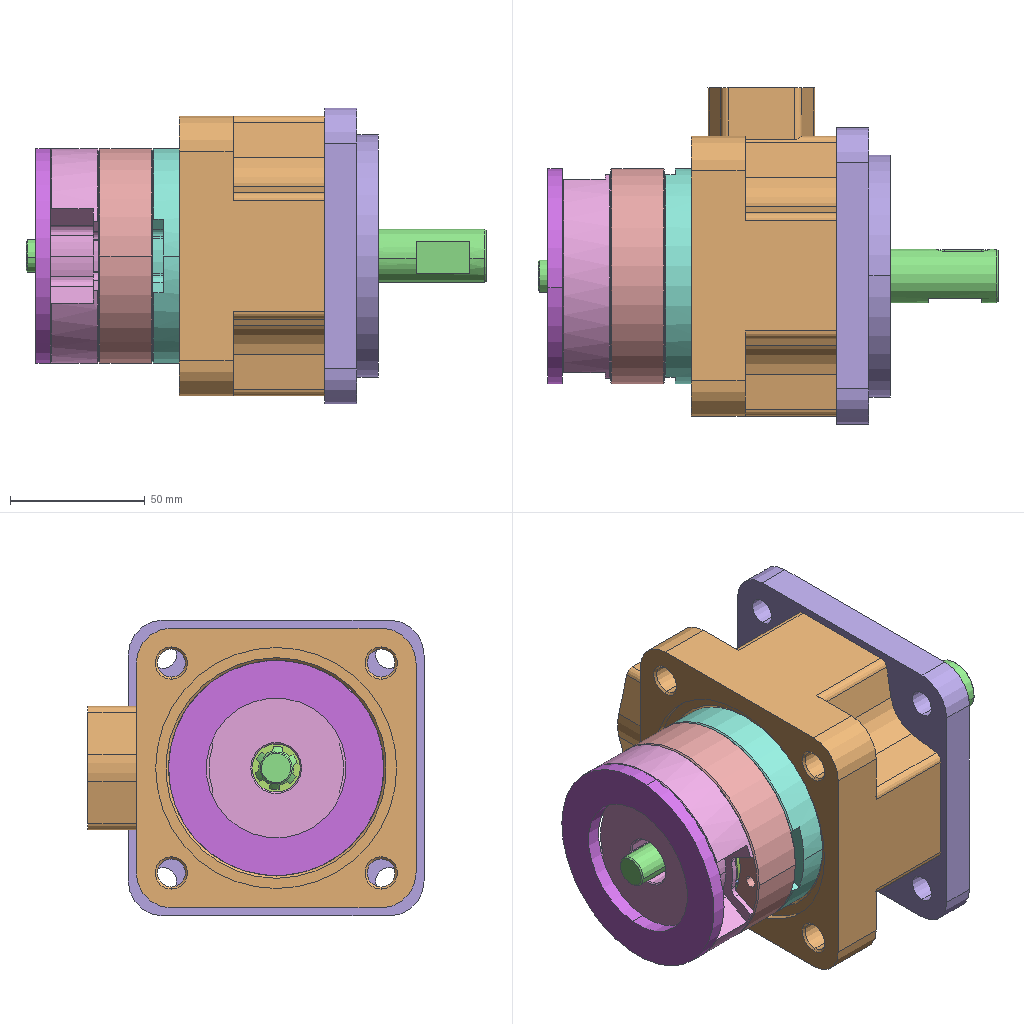Assembly | SolidWorks | 12 different items | 25 placed | box 171 x 125 x 110 mm
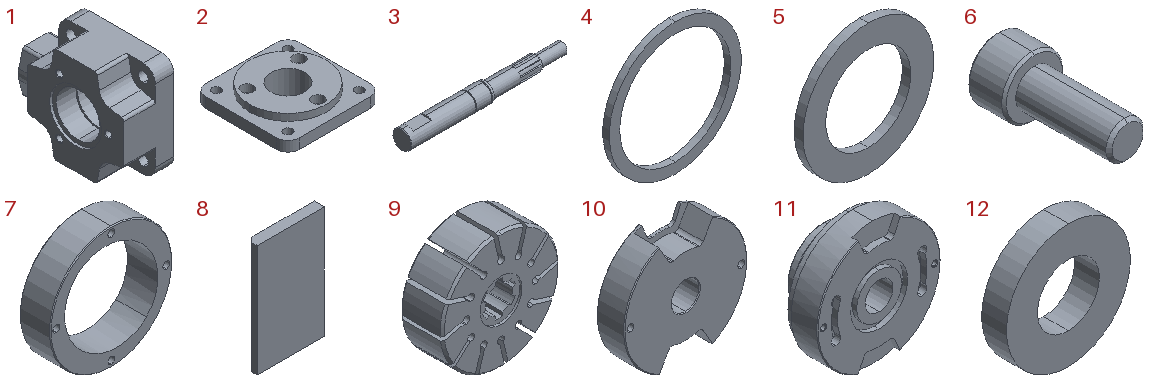Parts list (item | quantity | size | volume | features):
1 | x1 | 54 x 122 x 104 mm | 319990 mm3 | features ICE 11, HoleWzd 3, Chamfer 2, Extrusion 1, Fillet 1
2 | x1 | 110 x 110 x 29.8 mm | 163882 mm3 | features ICE 6, CirPattern 1, Extrusion 1
3 | x1 | 171 x 20 x 20 mm | 40308 mm3 | features ICE 9, Chamfer 2, Extrusion 1
4 | x1 | 55.8 x 2.75 x 55.8 mm | 1954 mm3 | features Extrusion 1
5 | x1 | 80 x 5.3 x 80 mm | 15385 mm3 | features Extrusion 1
6 | x3 | 13 x 28 x 13 mm | 1927 mm3 | features ICE 2, Chamfer 1, Extrusion 1, StudWizard 1
7 | x1 | 80 x 20 x 80 mm | 40998 mm3 | features ICE 2, Chamfer 1, Extrusion 1
8 | x12 | 12 x 1.8 x 20 mm | 425.6 mm3 | features Extrusion 1, ICE 1
9 | x1 | 56 x 20 x 56 mm | 39199 mm3 | features ICE 5, Chamfer 1, Extrusion 1
10 | x1 | 80 x 18 x 75.795 mm | 68506 mm3 | features ICE 6, Chamfer 2, Extrusion 1
11 | x1 | 80 x 36 x 80 mm | 99071 mm3 | features ICE 10, Chamfer 2, Extrusion 1, HoleWzd 1, MirrorPattern 1
12 | x1 | 40 x 8 x 40 mm | 4862 mm3 | features Extrusion 1, ICE 1
Mates (type | each side: item.copy, entity, surface, feature):
Coincident | assembly plane | assembly plane | 3 times
Concentric | assembly face | 3.1 face cylinder Boss-Extrude1
Concentric | 1.1 face cylinder Cut-Extrude6 | 3.1 face cylinder Boss-Extrude1
Concentric | assembly face | 1.1 face cylinder M12x1.25 Tapped Hole1
Concentric | assembly face | 7.1 face cylinder Boss-Extrude1
Concentric | 10.1 face cylinder Cut-Extrude4 | 3.1 face cylinder Boss-Extrude6
Concentric | 11.1 face cylinder Cut-Extrude1 | 3.1 face cylinder Boss-Extrude1
Concentric | 12.1 face cylinder Boss-Extrude1 | 3.1 face cylinder Boss-Extrude1
Concentric | 9.1 face cylinder Cut-Extrude2 | 3.1 face cylinder Boss-Extrude1
Coincident | 8.1 face plane Boss-Extrude2 | 9.1 face plane Boss-Extrude1
Coincident | 8.1 face plane Boss-Extrude2 | 9.1 face plane Cut-Extrude5
Coincident | 7.1 face plane Boss-Extrude1 | 9.1 face plane Boss-Extrude1
Concentric | 7.1 face cylinder Cut-Extrude2 | 11.1 face cylinder M4 Tapped Hole1 | 2 times
Concentric | 7.1 face cylinder Cut-Extrude2 | 10.1 face cylinder Cut-Extrude1
Coincident | 7.1 face plane Boss-Extrude1 | 10.1 face plane Boss-Extrude1
Coincident | 7.1 face plane Boss-Extrude1 | 11.1 face plane Boss-Extrude1
Concentric | assembly face | 10.1 face cylinder Cut-Extrude1
Coincident | assembly face | 10.1 face plane Boss-Extrude1
Coincident | assembly face | 1.1 face plane Boss-Extrude1
Concentric | 3.1 face cylinder Boss-Extrude1 | 2.1 face cylinder Cut-Extrude2
Concentric | 1.1 face cylinder M8 Tapped Hole1 | 2.1 face cylinder CirPattern1
Coincident | 1.1 face plane Boss-Extrude2 | 2.1 face plane Boss-Extrude1
Coincident | assembly face | 3.1 face plane Boss-Extrude7
Coincident | 9.1 face plane Cut-Extrude2 | 3.1 face plane Cut-Extrude1
Coincident | 12.1 face plane Boss-Extrude1 | 2.1 face plane Boss-Extrude2
Concentric | 3.1 face cylinder Boss-Extrude1 | assembly face | 6 times
Concentric | 3.1 face cylinder Boss-Extrude1 | 4.1 face cylinder Boss-Extrude1
Concentric | 4.1 face cylinder Boss-Extrude1 | assembly face
Coincident | 2.1 face plane Boss-Extrude1 | 4.1 face plane Boss-Extrude1
Coincident | 11.1 face plane Boss-Extrude3 | assembly face
Coincident | assembly face | assembly face | 4 times
Coincident | 1.1 face plane Cut-Extrude6 | assembly face
Coincident | 2.1 face plane Boss-Extrude3 | assembly face
Tangent | 9.1 face cylinder Boss-Extrude1 | 8.2 face plane Boss-Extrude2
Concentric | assembly face | assembly face
Concentric | 2.1 face cylinder CirPattern1 | 6.1 face cylinder Boss-Extrude1
Coincident | 2.1 face plane Boss-Extrude2 | 6.1 face plane Boss-Extrude2
Concentric | 3.1 face cylinder Boss-Extrude1 | 5.1 face cylinder Boss-Extrude1
Coincident | 10.1 face plane Boss-Extrude1 | 5.1 face plane Boss-Extrude1